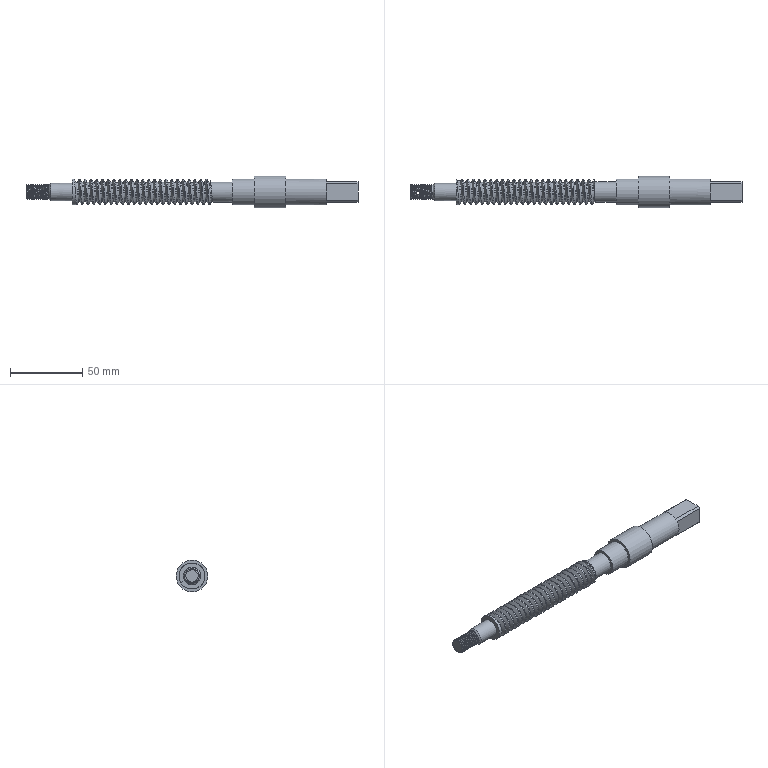Part | NX | features DATUM_CSYS 4, SKETCH 3, EXTRUDE 2, THREADS 2, CHAMFER 1, SWP104 1 | 1 solid | 46 faces | box 230 x 22 x 22 mm | volume 46800 mm3 | plane 18 | cylinder 17 | spline 10 | cone 1 | commonest cylinder face diameters 8.5 x4 10 x4 18 x3 14 x2 2.365 x1 12 x1